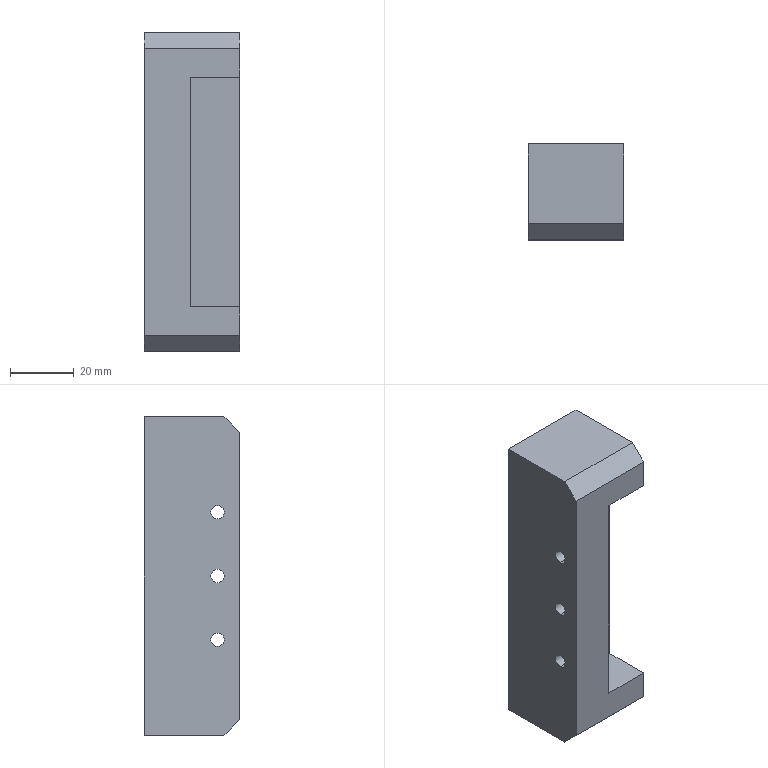Part | SolidWorks | features HoleWzd 2, Chamfer 1, Extrusion 1, ICE 1 | 1 solid | 30 faces | box 30 x 30 x 100 mm | volume 70744 mm3 | cylinder 12 | plane 12 | cone 6 | commonest cylinder face diameters 4.2 x6 6.8 x6
STEP:
#1=CARTESIAN_POINT('',(0.,-8.,22.1));
#2=VERTEX_POINT('',#1);
#3=CARTESIAN_POINT('',(0.,-8.,17.9));
#4=VERTEX_POINT('',#3);
#5=CARTESIAN_POINT('',(0.,-8.,20.));
#6=DIRECTION('',(1.,0.,0.));
#7=DIRECTION('',(0.,0.,-1.));
#8=AXIS2_PLACEMENT_3D('',#5,#6,#7);
#9=CIRCLE('',#8,2.1);
#10=EDGE_CURVE('',#2,#4,#9,.T.);
#11=ORIENTED_EDGE('',*,*,#10,.F.);
#12=CARTESIAN_POINT('',(14.5,-8.,22.1));
#13=VERTEX_POINT('',#12);
#14=CARTESIAN_POINT('',(14.5,-8.,22.1));
#15=DIRECTION('',(1.,0.,0.));
#16=VECTOR('',#15,1000.);
#17=LINE('',#14,#16);
#18=EDGE_CURVE('',#2,#13,#17,.T.);
#19=ORIENTED_EDGE('',*,*,#18,.T.);
#20=CARTESIAN_POINT('',(14.5,-8.,17.9));
#21=VERTEX_POINT('',#20);
#22=CARTESIAN_POINT('',(14.5,-8.,20.));
#23=DIRECTION('',(1.,0.,0.));
#24=DIRECTION('',(0.,0.,-1.));
#25=AXIS2_PLACEMENT_3D('',#22,#23,#24);
#26=CIRCLE('',#25,2.1);
#27=EDGE_CURVE('',#13,#21,#26,.T.);
#28=ORIENTED_EDGE('',*,*,#27,.T.);
#29=CARTESIAN_POINT('',(14.5,-8.,17.9));
#30=DIRECTION('',(1.,0.,0.));
#31=VECTOR('',#30,1000.);
#32=LINE('',#29,#31);
#33=EDGE_CURVE('',#4,#21,#32,.T.);
#34=ORIENTED_EDGE('',*,*,#33,.F.);
#35=EDGE_LOOP('',(#11,#19,#28,#34));
#36=FACE_OUTER_BOUND('',#35,.T.);
#37=CARTESIAN_POINT('',(14.5,-8.,20.));
#38=DIRECTION('',(1.,0.,0.));
#39=DIRECTION('',(0.,0.,-1.));
#40=AXIS2_PLACEMENT_3D('',#37,#38,#39);
#41=CYLINDRICAL_SURFACE('',#40,2.1);
#42=ADVANCED_FACE('',(#36),#41,.F.);
#43=CARTESIAN_POINT('',(0.,-8.,2.1));
#44=VERTEX_POINT('',#43);
#45=CARTESIAN_POINT('',(0.,-8.,-2.1));
#46=VERTEX_POINT('',#45);
#47=CARTESIAN_POINT('',(0.,-8.,0.));
#48=DIRECTION('',(1.,0.,0.));
#49=DIRECTION('',(0.,0.,-1.));
#50=AXIS2_PLACEMENT_3D('',#47,#48,#49);
#51=CIRCLE('',#50,2.1);
#52=EDGE_CURVE('',#44,#46,#51,.T.);
#53=ORIENTED_EDGE('',*,*,#52,.F.);
#54=CARTESIAN_POINT('',(14.5,-8.,2.1));
#55=VERTEX_POINT('',#54);
#56=CARTESIAN_POINT('',(14.5,-8.,2.1));
#57=DIRECTION('',(1.,0.,0.));
#58=VECTOR('',#57,1000.);
#59=LINE('',#56,#58);
#60=EDGE_CURVE('',#44,#55,#59,.T.);
#61=ORIENTED_EDGE('',*,*,#60,.T.);
#62=CARTESIAN_POINT('',(14.5,-8.,-2.1));
#63=VERTEX_POINT('',#62);
#64=CARTESIAN_POINT('',(14.5,-8.,0.));
#65=DIRECTION('',(1.,0.,0.));
#66=DIRECTION('',(0.,0.,-1.));
#67=AXIS2_PLACEMENT_3D('',#64,#65,#66);
#68=CIRCLE('',#67,2.1);
#69=EDGE_CURVE('',#55,#63,#68,.T.);
#70=ORIENTED_EDGE('',*,*,#69,.T.);
#71=CARTESIAN_POINT('',(14.5,-8.,-2.1));
#72=DIRECTION('',(1.,0.,0.));
#73=VECTOR('',#72,1000.);
#74=LINE('',#71,#73);
#75=EDGE_CURVE('',#46,#63,#74,.T.);
#76=ORIENTED_EDGE('',*,*,#75,.F.);
#77=EDGE_LOOP('',(#53,#61,#70,#76));
#78=FACE_OUTER_BOUND('',#77,.T.);
#79=CARTESIAN_POINT('',(14.5,-8.,0.));
#80=DIRECTION('',(1.,0.,0.));
#81=DIRECTION('',(0.,0.,-1.));
#82=AXIS2_PLACEMENT_3D('',#79,#80,#81);
#83=CYLINDRICAL_SURFACE('',#82,2.1);
#84=ADVANCED_FACE('',(#78),#83,.F.);
#85=CARTESIAN_POINT('',(0.,-8.,-17.9));
#86=VERTEX_POINT('',#85);
#87=CARTESIAN_POINT('',(0.,-8.,-22.1));
#88=VERTEX_POINT('',#87);
#89=CARTESIAN_POINT('',(0.,-8.,-20.));
#90=DIRECTION('',(1.,0.,0.));
#91=DIRECTION('',(0.,0.,-1.));
#92=AXIS2_PLACEMENT_3D('',#89,#90,#91);
#93=CIRCLE('',#92,2.1);
#94=EDGE_CURVE('',#86,#88,#93,.T.);
#95=ORIENTED_EDGE('',*,*,#94,.F.);
#96=CARTESIAN_POINT('',(14.5,-8.,-17.9));
#97=VERTEX_POINT('',#96);
#98=CARTESIAN_POINT('',(14.5,-8.,-17.9));
#99=DIRECTION('',(1.,0.,0.));
#100=VECTOR('',#99,1000.);
#101=LINE('',#98,#100);
#102=EDGE_CURVE('',#86,#97,#101,.T.);
#103=ORIENTED_EDGE('',*,*,#102,.T.);
#104=CARTESIAN_POINT('',(14.5,-8.,-22.1));
#105=VERTEX_POINT('',#104);
#106=CARTESIAN_POINT('',(14.5,-8.,-20.));
#107=DIRECTION('',(1.,0.,0.));
#108=DIRECTION('',(0.,0.,-1.));
#109=AXIS2_PLACEMENT_3D('',#106,#107,#108);
#110=CIRCLE('',#109,2.1);
#111=EDGE_CURVE('',#97,#105,#110,.T.);
#112=ORIENTED_EDGE('',*,*,#111,.T.);
#113=CARTESIAN_POINT('',(14.5,-8.,-22.1));
#114=DIRECTION('',(1.,0.,0.));
#115=VECTOR('',#114,1000.);
#116=LINE('',#113,#115);
#117=EDGE_CURVE('',#88,#105,#116,.T.);
#118=ORIENTED_EDGE('',*,*,#117,.F.);
#119=EDGE_LOOP('',(#95,#103,#112,#118));
#120=FACE_OUTER_BOUND('',#119,.T.);
#121=CARTESIAN_POINT('',(14.5,-8.,-20.));
#122=DIRECTION('',(1.,0.,0.));
#123=DIRECTION('',(0.,0.,-1.));
#124=AXIS2_PLACEMENT_3D('',#121,#122,#123);
#125=CYLINDRICAL_SURFACE('',#124,2.1);
#126=ADVANCED_FACE('',(#120),#125,.F.);
#127=CARTESIAN_POINT('',(15.,5.,-3.4));
#128=VERTEX_POINT('',#127);
#129=CARTESIAN_POINT('',(15.,5.,3.4));
#130=VERTEX_POINT('',#129);
#131=CARTESIAN_POINT('',(15.,5.,0.));
#132=DIRECTION('',(0.,1.,0.));
#133=DIRECTION('',(0.,0.,1.));
#134=AXIS2_PLACEMENT_3D('',#131,#132,#133);
#135=CIRCLE('',#134,3.4);
#136=EDGE_CURVE('',#128,#130,#135,.T.);
#137=ORIENTED_EDGE('',*,*,#136,.F.);
#138=CARTESIAN_POINT('',(15.,15.,-3.4));
#139=VERTEX_POINT('',#138);
#140=CARTESIAN_POINT('',(15.,15.,-3.4));
#141=DIRECTION('',(0.,1.,0.));
#142=VECTOR('',#141,1000.);
#143=LINE('',#140,#142);
#144=EDGE_CURVE('',#128,#139,#143,.T.);
#145=ORIENTED_EDGE('',*,*,#144,.T.);
#146=CARTESIAN_POINT('',(15.,15.,3.4));
#147=VERTEX_POINT('',#146);
#148=CARTESIAN_POINT('',(15.,15.,0.));
#149=DIRECTION('',(0.,1.,0.));
#150=DIRECTION('',(0.,0.,1.));
#151=AXIS2_PLACEMENT_3D('',#148,#149,#150);
#152=CIRCLE('',#151,3.4);
#153=EDGE_CURVE('',#139,#147,#152,.T.);
#154=ORIENTED_EDGE('',*,*,#153,.T.);
#155=CARTESIAN_POINT('',(15.,15.,3.4));
#156=DIRECTION('',(0.,1.,0.));
#157=VECTOR('',#156,1000.);
#158=LINE('',#155,#157);
#159=EDGE_CURVE('',#130,#147,#158,.T.);
#160=ORIENTED_EDGE('',*,*,#159,.F.);
#161=EDGE_LOOP('',(#137,#145,#154,#160));
#162=FACE_OUTER_BOUND('',#161,.T.);
#163=CARTESIAN_POINT('',(15.,15.,0.));
#164=DIRECTION('',(0.,1.,0.));
#165=DIRECTION('',(0.,0.,1.));
#166=AXIS2_PLACEMENT_3D('',#163,#164,#165);
#167=CYLINDRICAL_SURFACE('',#166,3.4);
#168=ADVANCED_FACE('',(#162),#167,.F.);
#169=CARTESIAN_POINT('',(15.,2.957,0.));
#170=VERTEX_POINT('',#169);
#171=CARTESIAN_POINT('',(15.,5.,3.4));
#172=DIRECTION('',(0.,0.515,0.8572));
#173=VECTOR('',#172,1000.);
#174=LINE('',#171,#173);
#175=EDGE_CURVE('',#170,#130,#174,.T.);
#176=ORIENTED_EDGE('',*,*,#175,.F.);
#177=CARTESIAN_POINT('',(15.,5.,-3.4));
#178=DIRECTION('',(0.,0.515,-0.8572));
#179=VECTOR('',#178,1000.);
#180=LINE('',#177,#179);
#181=EDGE_CURVE('',#170,#128,#180,.T.);
#182=ORIENTED_EDGE('',*,*,#181,.T.);
#183=ORIENTED_EDGE('',*,*,#136,.T.);
#184=EDGE_LOOP('',(#176,#182,#183));
#185=FACE_OUTER_BOUND('',#184,.T.);
#186=CARTESIAN_POINT('',(15.,5.,0.));
#187=DIRECTION('',(0.,1.,0.));
#188=DIRECTION('',(0.,0.,1.));
#189=AXIS2_PLACEMENT_3D('',#186,#187,#188);
#190=CONICAL_SURFACE('',#189,3.4,1.03);
#191=ADVANCED_FACE('',(#185),#190,.F.);
#192=CARTESIAN_POINT('',(15.,5.,-28.4));
#193=VERTEX_POINT('',#192);
#194=CARTESIAN_POINT('',(15.,5.,-21.6));
#195=VERTEX_POINT('',#194);
#196=CARTESIAN_POINT('',(15.,5.,-25.));
#197=DIRECTION('',(0.,1.,0.));
#198=DIRECTION('',(0.,0.,1.));
#199=AXIS2_PLACEMENT_3D('',#196,#197,#198);
#200=CIRCLE('',#199,3.4);
#201=EDGE_CURVE('',#193,#195,#200,.T.);
#202=ORIENTED_EDGE('',*,*,#201,.F.);
#203=CARTESIAN_POINT('',(15.,15.,-28.4));
#204=VERTEX_POINT('',#203);
#205=CARTESIAN_POINT('',(15.,15.,-28.4));
#206=DIRECTION('',(0.,1.,0.));
#207=VECTOR('',#206,1000.);
#208=LINE('',#205,#207);
#209=EDGE_CURVE('',#193,#204,#208,.T.);
#210=ORIENTED_EDGE('',*,*,#209,.T.);
#211=CARTESIAN_POINT('',(15.,15.,-21.6));
#212=VERTEX_POINT('',#211);
#213=CARTESIAN_POINT('',(15.,15.,-25.));
#214=DIRECTION('',(0.,1.,0.));
#215=DIRECTION('',(0.,0.,1.));
#216=AXIS2_PLACEMENT_3D('',#213,#214,#215);
#217=CIRCLE('',#216,3.4);
#218=EDGE_CURVE('',#204,#212,#217,.T.);
#219=ORIENTED_EDGE('',*,*,#218,.T.);
#220=CARTESIAN_POINT('',(15.,15.,-21.6));
#221=DIRECTION('',(0.,1.,0.));
#222=VECTOR('',#221,1000.);
#223=LINE('',#220,#222);
#224=EDGE_CURVE('',#195,#212,#223,.T.);
#225=ORIENTED_EDGE('',*,*,#224,.F.);
#226=EDGE_LOOP('',(#202,#210,#219,#225));
#227=FACE_OUTER_BOUND('',#226,.T.);
#228=CARTESIAN_POINT('',(15.,15.,-25.));
#229=DIRECTION('',(0.,1.,0.));
#230=DIRECTION('',(0.,0.,1.));
#231=AXIS2_PLACEMENT_3D('',#228,#229,#230);
#232=CYLINDRICAL_SURFACE('',#231,3.4);
#233=ADVANCED_FACE('',(#227),#232,.F.);
#234=CARTESIAN_POINT('',(15.,2.957,-25.));
#235=VERTEX_POINT('',#234);
#236=CARTESIAN_POINT('',(15.,5.,-21.6));
#237=DIRECTION('',(0.,0.515,0.8572));
#238=VECTOR('',#237,1000.);
#239=LINE('',#236,#238);
#240=EDGE_CURVE('',#235,#195,#239,.T.);
#241=ORIENTED_EDGE('',*,*,#240,.F.);
#242=CARTESIAN_POINT('',(15.,5.,-28.4));
#243=DIRECTION('',(0.,0.515,-0.8572));
#244=VECTOR('',#243,1000.);
#245=LINE('',#242,#244);
#246=EDGE_CURVE('',#235,#193,#245,.T.);
#247=ORIENTED_EDGE('',*,*,#246,.T.);
#248=ORIENTED_EDGE('',*,*,#201,.T.);
#249=EDGE_LOOP('',(#241,#247,#248));
#250=FACE_OUTER_BOUND('',#249,.T.);
#251=CARTESIAN_POINT('',(15.,5.,-25.));
#252=DIRECTION('',(0.,1.,0.));
#253=DIRECTION('',(0.,0.,1.));
#254=AXIS2_PLACEMENT_3D('',#251,#252,#253);
#255=CONICAL_SURFACE('',#254,3.4,1.03);
#256=ADVANCED_FACE('',(#250),#255,.F.);
#257=CARTESIAN_POINT('',(15.,5.,21.6));
#258=VERTEX_POINT('',#257);
#259=CARTESIAN_POINT('',(15.,5.,28.4));
#260=VERTEX_POINT('',#259);
#261=CARTESIAN_POINT('',(15.,5.,25.));
#262=DIRECTION('',(0.,1.,0.));
#263=DIRECTION('',(0.,0.,1.));
#264=AXIS2_PLACEMENT_3D('',#261,#262,#263);
#265=CIRCLE('',#264,3.4);
#266=EDGE_CURVE('',#258,#260,#265,.T.);
#267=ORIENTED_EDGE('',*,*,#266,.F.);
#268=CARTESIAN_POINT('',(15.,15.,21.6));
#269=VERTEX_POINT('',#268);
#270=CARTESIAN_POINT('',(15.,15.,21.6));
#271=DIRECTION('',(0.,1.,0.));
#272=VECTOR('',#271,1000.);
#273=LINE('',#270,#272);
#274=EDGE_CURVE('',#258,#269,#273,.T.);
#275=ORIENTED_EDGE('',*,*,#274,.T.);
#276=CARTESIAN_POINT('',(15.,15.,28.4));
#277=VERTEX_POINT('',#276);
#278=CARTESIAN_POINT('',(15.,15.,25.));
#279=DIRECTION('',(0.,1.,0.));
#280=DIRECTION('',(0.,0.,1.));
#281=AXIS2_PLACEMENT_3D('',#278,#279,#280);
#282=CIRCLE('',#281,3.4);
#283=EDGE_CURVE('',#269,#277,#282,.T.);
#284=ORIENTED_EDGE('',*,*,#283,.T.);
#285=CARTESIAN_POINT('',(15.,15.,28.4));
#286=DIRECTION('',(0.,1.,0.));
#287=VECTOR('',#286,1000.);
#288=LINE('',#285,#287);
#289=EDGE_CURVE('',#260,#277,#288,.T.);
#290=ORIENTED_EDGE('',*,*,#289,.F.);
#291=EDGE_LOOP('',(#267,#275,#284,#290));
#292=FACE_OUTER_BOUND('',#291,.T.);
#293=CARTESIAN_POINT('',(15.,15.,25.));
#294=DIRECTION('',(0.,1.,0.));
#295=DIRECTION('',(0.,0.,1.));
#296=AXIS2_PLACEMENT_3D('',#293,#294,#295);
#297=CYLINDRICAL_SURFACE('',#296,3.4);
#298=ADVANCED_FACE('',(#292),#297,.F.);
#299=CARTESIAN_POINT('',(15.,2.957,25.));
#300=VERTEX_POINT('',#299);
#301=CARTESIAN_POINT('',(15.,5.,28.4));
#302=DIRECTION('',(0.,0.515,0.8572));
#303=VECTOR('',#302,1000.);
#304=LINE('',#301,#303);
#305=EDGE_CURVE('',#300,#260,#304,.T.);
#306=ORIENTED_EDGE('',*,*,#305,.F.);
#307=CARTESIAN_POINT('',(15.,5.,21.6));
#308=DIRECTION('',(0.,0.515,-0.8572));
#309=VECTOR('',#308,1000.);
#310=LINE('',#307,#309);
#311=EDGE_CURVE('',#300,#258,#310,.T.);
#312=ORIENTED_EDGE('',*,*,#311,.T.);
#313=ORIENTED_EDGE('',*,*,#266,.T.);
#314=EDGE_LOOP('',(#306,#312,#313));
#315=FACE_OUTER_BOUND('',#314,.T.);
#316=CARTESIAN_POINT('',(15.,5.,25.));
#317=DIRECTION('',(0.,1.,0.));
#318=DIRECTION('',(0.,0.,1.));
#319=AXIS2_PLACEMENT_3D('',#316,#317,#318);
#320=CONICAL_SURFACE('',#319,3.4,1.03);
#321=ADVANCED_FACE('',(#315),#320,.F.);
#322=CARTESIAN_POINT('',(30.,-10.,-50.));
#323=VERTEX_POINT('',#322);
#324=CARTESIAN_POINT('',(30.,15.,-50.));
#325=VERTEX_POINT('',#324);
#326=CARTESIAN_POINT('',(30.,15.,-50.));
#327=DIRECTION('',(0.,1.,0.));
#328=VECTOR('',#327,1000.);
#329=LINE('',#326,#328);
#330=EDGE_CURVE('',#323,#325,#329,.T.);
#331=ORIENTED_EDGE('',*,*,#330,.F.);
#332=CARTESIAN_POINT('',(0.,-10.,-50.));
#333=VERTEX_POINT('',#332);
#334=CARTESIAN_POINT('',(30.,-10.,-50.));
#335=DIRECTION('',(-1.,0.,0.));
#336=VECTOR('',#335,1000.);
#337=LINE('',#334,#336);
#338=EDGE_CURVE('',#323,#333,#337,.T.);
#339=ORIENTED_EDGE('',*,*,#338,.T.);
#340=CARTESIAN_POINT('',(0.,15.,-50.));
#341=VERTEX_POINT('',#340);
#342=CARTESIAN_POINT('',(0.,15.,-50.));
#343=DIRECTION('',(0.,1.,0.));
#344=VECTOR('',#343,1000.);
#345=LINE('',#342,#344);
#346=EDGE_CURVE('',#333,#341,#345,.T.);
#347=ORIENTED_EDGE('',*,*,#346,.T.);
#348=CARTESIAN_POINT('',(30.,15.,-50.));
#349=DIRECTION('',(-1.,0.,0.));
#350=VECTOR('',#349,1000.);
#351=LINE('',#348,#350);
#352=EDGE_CURVE('',#325,#341,#351,.T.);
#353=ORIENTED_EDGE('',*,*,#352,.F.);
#354=EDGE_LOOP('',(#331,#339,#347,#353));
#355=FACE_OUTER_BOUND('',#354,.T.);
#356=CARTESIAN_POINT('',(30.,15.,-50.));
#357=DIRECTION('',(0.,0.,1.));
#358=DIRECTION('',(0.,-1.,0.));
#359=AXIS2_PLACEMENT_3D('',#356,#357,#358);
#360=PLANE('',#359);
#361=ADVANCED_FACE('',(#355),#360,.F.);
#362=CARTESIAN_POINT('',(15.,15.,0.));
#363=DIRECTION('',(0.,1.,0.));
#364=DIRECTION('',(0.,0.,1.));
#365=AXIS2_PLACEMENT_3D('',#362,#363,#364);
#366=CIRCLE('',#365,3.4);
#367=EDGE_CURVE('',#147,#139,#366,.T.);
#368=ORIENTED_EDGE('',*,*,#367,.F.);
#369=ORIENTED_EDGE('',*,*,#153,.F.);
#370=EDGE_LOOP('',(#368,#369));
#371=FACE_BOUND('',#370,.T.);
#372=CARTESIAN_POINT('',(15.,15.,-25.));
#373=DIRECTION('',(0.,1.,0.));
#374=DIRECTION('',(0.,0.,1.));
#375=AXIS2_PLACEMENT_3D('',#372,#373,#374);
#376=CIRCLE('',#375,3.4);
#377=EDGE_CURVE('',#212,#204,#376,.T.);
#378=ORIENTED_EDGE('',*,*,#377,.F.);
#379=ORIENTED_EDGE('',*,*,#218,.F.);
#380=EDGE_LOOP('',(#378,#379));
#381=FACE_BOUND('',#380,.T.);
#382=CARTESIAN_POINT('',(15.,15.,25.));
#383=DIRECTION('',(0.,1.,0.));
#384=DIRECTION('',(0.,0.,1.));
#385=AXIS2_PLACEMENT_3D('',#382,#383,#384);
#386=CIRCLE('',#385,3.4);
#387=EDGE_CURVE('',#277,#269,#386,.T.);
#388=ORIENTED_EDGE('',*,*,#387,.F.);
#389=ORIENTED_EDGE('',*,*,#283,.F.);
#390=EDGE_LOOP('',(#388,#389));
#391=FACE_BOUND('',#390,.T.);
#392=CARTESIAN_POINT('',(0.,15.,50.));
#393=VERTEX_POINT('',#392);
#394=CARTESIAN_POINT('',(0.,15.,50.));
#395=DIRECTION('',(0.,0.,1.));
#396=VECTOR('',#395,1000.);
#397=LINE('',#394,#396);
#398=EDGE_CURVE('',#341,#393,#397,.T.);
#399=ORIENTED_EDGE('',*,*,#398,.T.);
#400=CARTESIAN_POINT('',(30.,15.,50.));
#401=VERTEX_POINT('',#400);
#402=CARTESIAN_POINT('',(30.,15.,50.));
#403=DIRECTION('',(-1.,0.,0.));
#404=VECTOR('',#403,1000.);
#405=LINE('',#402,#404);
#406=EDGE_CURVE('',#401,#393,#405,.T.);
#407=ORIENTED_EDGE('',*,*,#406,.F.);
#408=CARTESIAN_POINT('',(30.,15.,50.));
#409=DIRECTION('',(0.,0.,1.));
#410=VECTOR('',#409,1000.);
#411=LINE('',#408,#410);
#412=EDGE_CURVE('',#325,#401,#411,.T.);
#413=ORIENTED_EDGE('',*,*,#412,.F.);
#414=ORIENTED_EDGE('',*,*,#352,.T.);
#415=EDGE_LOOP('',(#399,#407,#413,#414));
#416=FACE_OUTER_BOUND('',#415,.T.);
#417=CARTESIAN_POINT('',(30.,15.,50.));
#418=DIRECTION('',(0.,-1.,0.));
#419=DIRECTION('',(0.,0.,-1.));
#420=AXIS2_PLACEMENT_3D('',#417,#418,#419);
#421=PLANE('',#420);
#422=ADVANCED_FACE('',(#371,#381,#391,#416),#421,.F.);
#423=CARTESIAN_POINT('',(0.,-10.,50.));
#424=VERTEX_POINT('',#423);
#425=CARTESIAN_POINT('',(0.,15.,50.));
#426=DIRECTION('',(0.,-1.,0.));
#427=VECTOR('',#426,1000.);
#428=LINE('',#425,#427);
#429=EDGE_CURVE('',#393,#424,#428,.T.);
#430=ORIENTED_EDGE('',*,*,#429,.T.);
#431=CARTESIAN_POINT('',(30.,-10.,50.));
#432=VERTEX_POINT('',#431);
#433=CARTESIAN_POINT('',(30.,-10.,50.));
#434=DIRECTION('',(1.,0.,0.));
#435=VECTOR('',#434,1000.);
#436=LINE('',#433,#435);
#437=EDGE_CURVE('',#424,#432,#436,.T.);
#438=ORIENTED_EDGE('',*,*,#437,.T.);
#439=CARTESIAN_POINT('',(30.,15.,50.));
#440=DIRECTION('',(0.,-1.,0.));
#441=VECTOR('',#440,1000.);
#442=LINE('',#439,#441);
#443=EDGE_CURVE('',#401,#432,#442,.T.);
#444=ORIENTED_EDGE('',*,*,#443,.F.);
#445=ORIENTED_EDGE('',*,*,#406,.T.);
#446=EDGE_LOOP('',(#430,#438,#444,#445));
#447=FACE_OUTER_BOUND('',#446,.T.);
#448=CARTESIAN_POINT('',(30.,15.,50.));
#449=DIRECTION('',(0.,0.,-1.));
#450=DIRECTION('',(0.,1.,0.));
#451=AXIS2_PLACEMENT_3D('',#448,#449,#450);
#452=PLANE('',#451);
#453=ADVANCED_FACE('',(#447),#452,.F.);
#454=CARTESIAN_POINT('',(30.,-15.,45.));
#455=VERTEX_POINT('',#454);
#456=CARTESIAN_POINT('',(30.,-15.,36.));
#457=VERTEX_POINT('',#456);
#458=CARTESIAN_POINT('',(30.,-15.,50.));
#459=DIRECTION('',(0.,0.,-1.));
#460=VECTOR('',#459,1000.);
#461=LINE('',#458,#460);
#462=EDGE_CURVE('',#455,#457,#461,.T.);
#463=ORIENTED_EDGE('',*,*,#462,.F.);
#464=CARTESIAN_POINT('',(0.,-15.,45.));
#465=VERTEX_POINT('',#464);
#466=CARTESIAN_POINT('',(30.,-15.,45.));
#467=DIRECTION('',(-1.,0.,0.));
#468=VECTOR('',#467,1000.);
#469=LINE('',#466,#468);
#470=EDGE_CURVE('',#455,#465,#469,.T.);
#471=ORIENTED_EDGE('',*,*,#470,.T.);
#472=CARTESIAN_POINT('',(0.,-15.,-45.));
#473=VERTEX_POINT('',#472);
#474=CARTESIAN_POINT('',(0.,-15.,50.));
#475=DIRECTION('',(0.,0.,-1.));
#476=VECTOR('',#475,1000.);
#477=LINE('',#474,#476);
#478=EDGE_CURVE('',#465,#473,#477,.T.);
#479=ORIENTED_EDGE('',*,*,#478,.T.);
#480=CARTESIAN_POINT('',(30.,-15.,-45.));
#481=VERTEX_POINT('',#480);
#482=CARTESIAN_POINT('',(30.,-15.,-45.));
#483=DIRECTION('',(1.,0.,0.));
#484=VECTOR('',#483,1000.);
#485=LINE('',#482,#484);
#486=EDGE_CURVE('',#473,#481,#485,.T.);
#487=ORIENTED_EDGE('',*,*,#486,.T.);
#488=CARTESIAN_POINT('',(30.,-15.,-36.));
#489=VERTEX_POINT('',#488);
#490=CARTESIAN_POINT('',(30.,-15.,50.));
#491=DIRECTION('',(0.,0.,-1.));
#492=VECTOR('',#491,1000.);
#493=LINE('',#490,#492);
#494=EDGE_CURVE('',#489,#481,#493,.T.);
#495=ORIENTED_EDGE('',*,*,#494,.F.);
#496=CARTESIAN_POINT('',(14.5,-15.,-36.));
#497=VERTEX_POINT('',#496);
#498=CARTESIAN_POINT('',(14.5,-15.,-36.));
#499=DIRECTION('',(1.,0.,0.));
#500=VECTOR('',#499,1000.);
#501=LINE('',#498,#500);
#502=EDGE_CURVE('',#497,#489,#501,.T.);
#503=ORIENTED_EDGE('',*,*,#502,.F.);
#504=CARTESIAN_POINT('',(14.5,-15.,36.));
#505=VERTEX_POINT('',#504);
#506=CARTESIAN_POINT('',(14.5,-15.,36.));
#507=DIRECTION('',(0.,0.,-1.));
#508=VECTOR('',#507,1000.);
#509=LINE('',#506,#508);
#510=EDGE_CURVE('',#505,#497,#509,.T.);
#511=ORIENTED_EDGE('',*,*,#510,.F.);
#512=CARTESIAN_POINT('',(14.5,-15.,36.));
#513=DIRECTION('',(1.,0.,0.));
#514=VECTOR('',#513,1000.);
#515=LINE('',#512,#514);
#516=EDGE_CURVE('',#505,#457,#515,.T.);
#517=ORIENTED_EDGE('',*,*,#516,.T.);
#518=EDGE_LOOP('',(#463,#471,#479,#487,#495,#503,#511,#517));
#519=FACE_OUTER_BOUND('',#518,.T.);
#520=CARTESIAN_POINT('',(30.,-15.,50.));
#521=DIRECTION('',(0.,1.,0.));
#522=DIRECTION('',(0.,0.,1.));
#523=AXIS2_PLACEMENT_3D('',#520,#521,#522);
#524=PLANE('',#523);
#525=ADVANCED_FACE('',(#519),#524,.F.);
#526=ORIENTED_EDGE('',*,*,#443,.T.);
#527=CARTESIAN_POINT('',(30.,-30.,30.));
#528=DIRECTION('',(0.,-0.7071,-0.7071));
#529=VECTOR('',#528,1000.);
#530=LINE('',#527,#529);
#531=EDGE_CURVE('',#432,#455,#530,.T.);
#532=ORIENTED_EDGE('',*,*,#531,.T.);
#533=ORIENTED_EDGE('',*,*,#462,.T.);
#534=CARTESIAN_POINT('',(30.,0.,36.));
#535=VERTEX_POINT('',#534);
#536=CARTESIAN_POINT('',(30.,-15.,36.));
#537=DIRECTION('',(0.,-1.,0.));
#538=VECTOR('',#537,1000.);
#539=LINE('',#536,#538);
#540=EDGE_CURVE('',#535,#457,#539,.T.);
#541=ORIENTED_EDGE('',*,*,#540,.F.);
#542=CARTESIAN_POINT('',(30.,0.,-36.));
#543=VERTEX_POINT('',#542);
#544=CARTESIAN_POINT('',(30.,0.,36.));
#545=DIRECTION('',(0.,0.,1.));
#546=VECTOR('',#545,1000.);
#547=LINE('',#544,#546);
#548=EDGE_CURVE('',#543,#535,#547,.T.);
#549=ORIENTED_EDGE('',*,*,#548,.F.);
#550=CARTESIAN_POINT('',(30.,-15.,-36.));
#551=DIRECTION('',(0.,1.,0.));
#552=VECTOR('',#551,1000.);
#553=LINE('',#550,#552);
#554=EDGE_CURVE('',#489,#543,#553,.T.);
#555=ORIENTED_EDGE('',*,*,#554,.F.);
#556=ORIENTED_EDGE('',*,*,#494,.T.);
#557=CARTESIAN_POINT('',(30.,-30.,-30.));
#558=DIRECTION('',(0.,0.7071,-0.7071));
#559=VECTOR('',#558,1000.);
#560=LINE('',#557,#559);
#561=EDGE_CURVE('',#481,#323,#560,.T.);
#562=ORIENTED_EDGE('',*,*,#561,.T.);
#563=ORIENTED_EDGE('',*,*,#330,.T.);
#564=ORIENTED_EDGE('',*,*,#412,.T.);
#565=EDGE_LOOP('',(#526,#532,#533,#541,#549,#555,#556,#562,#563,#564));
#566=FACE_OUTER_BOUND('',#565,.T.);
#567=CARTESIAN_POINT('',(30.,0.,0.));
#568=DIRECTION('',(1.,0.,0.));
#569=DIRECTION('',(0.,0.,-1.));
#570=AXIS2_PLACEMENT_3D('',#567,#568,#569);
#571=PLANE('',#570);
#572=ADVANCED_FACE('',(#566),#571,.T.);
#573=CARTESIAN_POINT('',(0.,-8.,20.));
#574=DIRECTION('',(1.,0.,0.));
#575=DIRECTION('',(0.,0.,-1.));
#576=AXIS2_PLACEMENT_3D('',#573,#574,#575);
#577=CIRCLE('',#576,2.1);
#578=EDGE_CURVE('',#4,#2,#577,.T.);
#579=ORIENTED_EDGE('',*,*,#578,.T.);
#580=ORIENTED_EDGE('',*,*,#10,.T.);
#581=EDGE_LOOP('',(#579,#580));
#582=FACE_BOUND('',#581,.T.);
#583=CARTESIAN_POINT('',(0.,-8.,0.));
#584=DIRECTION('',(1.,0.,0.));
#585=DIRECTION('',(0.,0.,-1.));
#586=AXIS2_PLACEMENT_3D('',#583,#584,#585);
#587=CIRCLE('',#586,2.1);
#588=EDGE_CURVE('',#46,#44,#587,.T.);
#589=ORIENTED_EDGE('',*,*,#588,.T.);
#590=ORIENTED_EDGE('',*,*,#52,.T.);
#591=EDGE_LOOP('',(#589,#590));
#592=FACE_BOUND('',#591,.T.);
#593=CARTESIAN_POINT('',(0.,-8.,-20.));
#594=DIRECTION('',(1.,0.,0.));
#595=DIRECTION('',(0.,0.,-1.));
#596=AXIS2_PLACEMENT_3D('',#593,#594,#595);
#597=CIRCLE('',#596,2.1);
#598=EDGE_CURVE('',#88,#86,#597,.T.);
#599=ORIENTED_EDGE('',*,*,#598,.T.);
#600=ORIENTED_EDGE('',*,*,#94,.T.);
#601=EDGE_LOOP('',(#599,#600));
#602=FACE_BOUND('',#601,.T.);
#603=ORIENTED_EDGE('',*,*,#478,.F.);
#604=CARTESIAN_POINT('',(0.,-15.,45.));
#605=DIRECTION('',(0.,0.7071,0.7071));
#606=VECTOR('',#605,1000.);
#607=LINE('',#604,#606);
#608=EDGE_CURVE('',#465,#424,#607,.T.);
#609=ORIENTED_EDGE('',*,*,#608,.T.);
#610=ORIENTED_EDGE('',*,*,#429,.F.);
#611=ORIENTED_EDGE('',*,*,#398,.F.);
#612=ORIENTED_EDGE('',*,*,#346,.F.);
#613=CARTESIAN_POINT('',(0.,-10.,-50.));
#614=DIRECTION('',(0.,-0.7071,0.7071));
#615=VECTOR('',#614,1000.);
#616=LINE('',#613,#615);
#617=EDGE_CURVE('',#333,#473,#616,.T.);
#618=ORIENTED_EDGE('',*,*,#617,.T.);
#619=EDGE_LOOP('',(#603,#609,#610,#611,#612,#618));
#620=FACE_OUTER_BOUND('',#619,.T.);
#621=CARTESIAN_POINT('',(0.,0.,0.));
#622=DIRECTION('',(1.,0.,0.));
#623=DIRECTION('',(0.,0.,-1.));
#624=AXIS2_PLACEMENT_3D('',#621,#622,#623);
#625=PLANE('',#624);
#626=ADVANCED_FACE('',(#582,#592,#602,#620),#625,.F.);
#627=ORIENTED_EDGE('',*,*,#540,.T.);
#628=ORIENTED_EDGE('',*,*,#516,.F.);
#629=CARTESIAN_POINT('',(14.5,0.,36.));
#630=VERTEX_POINT('',#629);
#631=CARTESIAN_POINT('',(14.5,-15.,36.));
#632=DIRECTION('',(0.,-1.,0.));
#633=VECTOR('',#632,1000.);
#634=LINE('',#631,#633);
#635=EDGE_CURVE('',#630,#505,#634,.T.);
#636=ORIENTED_EDGE('',*,*,#635,.F.);
#637=CARTESIAN_POINT('',(14.5,0.,36.));
#638=DIRECTION('',(1.,0.,0.));
#639=VECTOR('',#638,1000.);
#640=LINE('',#637,#639);
#641=EDGE_CURVE('',#630,#535,#640,.T.);
#642=ORIENTED_EDGE('',*,*,#641,.T.);
#643=EDGE_LOOP('',(#627,#628,#636,#642));
#644=FACE_OUTER_BOUND('',#643,.T.);
#645=CARTESIAN_POINT('',(14.5,-15.,36.));
#646=DIRECTION('',(0.,0.,1.));
#647=DIRECTION('',(1.,0.,0.));
#648=AXIS2_PLACEMENT_3D('',#645,#646,#647);
#649=PLANE('',#648);
#650=ADVANCED_FACE('',(#644),#649,.F.);
#651=ORIENTED_EDGE('',*,*,#548,.T.);
#652=ORIENTED_EDGE('',*,*,#641,.F.);
#653=CARTESIAN_POINT('',(14.5,0.,-36.));
#654=VERTEX_POINT('',#653);
#655=CARTESIAN_POINT('',(14.5,0.,36.));
#656=DIRECTION('',(0.,0.,1.));
#657=VECTOR('',#656,1000.);
#658=LINE('',#655,#657);
#659=EDGE_CURVE('',#654,#630,#658,.T.);
#660=ORIENTED_EDGE('',*,*,#659,.F.);
#661=CARTESIAN_POINT('',(14.5,0.,-36.));
#662=DIRECTION('',(1.,0.,0.));
#663=VECTOR('',#662,1000.);
#664=LINE('',#661,#663);
#665=EDGE_CURVE('',#654,#543,#664,.T.);
#666=ORIENTED_EDGE('',*,*,#665,.T.);
#667=EDGE_LOOP('',(#651,#652,#660,#666));
#668=FACE_OUTER_BOUND('',#667,.T.);
#669=CARTESIAN_POINT('',(14.5,0.,36.));
#670=DIRECTION('',(0.,1.,0.));
#671=DIRECTION('',(0.,0.,1.));
#672=AXIS2_PLACEMENT_3D('',#669,#670,#671);
#673=PLANE('',#672);
#674=ADVANCED_FACE('',(#668),#673,.F.);
#675=ORIENTED_EDGE('',*,*,#554,.T.);
#676=ORIENTED_EDGE('',*,*,#665,.F.);
#677=CARTESIAN_POINT('',(14.5,-15.,-36.));
#678=DIRECTION('',(0.,1.,0.));
#679=VECTOR('',#678,1000.);
#680=LINE('',#677,#679);
#681=EDGE_CURVE('',#497,#654,#680,.T.);
#682=ORIENTED_EDGE('',*,*,#681,.F.);
#683=ORIENTED_EDGE('',*,*,#502,.T.);
#684=EDGE_LOOP('',(#675,#676,#682,#683));
#685=FACE_OUTER_BOUND('',#684,.T.);
#686=CARTESIAN_POINT('',(14.5,-15.,-36.));
#687=DIRECTION('',(0.,0.,-1.));
#688=DIRECTION('',(0.,1.,0.));
#689=AXIS2_PLACEMENT_3D('',#686,#687,#688);
#690=PLANE('',#689);
#691=ADVANCED_FACE('',(#685),#690,.F.);
#692=CARTESIAN_POINT('',(14.5,-8.,20.));
#693=DIRECTION('',(1.,0.,0.));
#694=DIRECTION('',(0.,0.,-1.));
#695=AXIS2_PLACEMENT_3D('',#692,#693,#694);
#696=CIRCLE('',#695,2.1);
#697=EDGE_CURVE('',#21,#13,#696,.T.);
#698=ORIENTED_EDGE('',*,*,#697,.F.);
#699=ORIENTED_EDGE('',*,*,#27,.F.);
#700=EDGE_LOOP('',(#698,#699));
#701=FACE_BOUND('',#700,.T.);
#702=CARTESIAN_POINT('',(14.5,-8.,0.));
#703=DIRECTION('',(1.,0.,0.));
#704=DIRECTION('',(0.,0.,-1.));
#705=AXIS2_PLACEMENT_3D('',#702,#703,#704);
#706=CIRCLE('',#705,2.1);
#707=EDGE_CURVE('',#63,#55,#706,.T.);
#708=ORIENTED_EDGE('',*,*,#707,.F.);
#709=ORIENTED_EDGE('',*,*,#69,.F.);
#710=EDGE_LOOP('',(#708,#709));
#711=FACE_BOUND('',#710,.T.);
#712=CARTESIAN_POINT('',(14.5,-8.,-20.));
#713=DIRECTION('',(1.,0.,0.));
#714=DIRECTION('',(0.,0.,-1.));
#715=AXIS2_PLACEMENT_3D('',#712,#713,#714);
#716=CIRCLE('',#715,2.1);
#717=EDGE_CURVE('',#105,#97,#716,.T.);
#718=ORIENTED_EDGE('',*,*,#717,.F.);
#719=ORIENTED_EDGE('',*,*,#111,.F.);
#720=EDGE_LOOP('',(#718,#719));
#721=FACE_BOUND('',#720,.T.);
#722=ORIENTED_EDGE('',*,*,#635,.T.);
#723=ORIENTED_EDGE('',*,*,#510,.T.);
#724=ORIENTED_EDGE('',*,*,#681,.T.);
#725=ORIENTED_EDGE('',*,*,#659,.T.);
#726=EDGE_LOOP('',(#722,#723,#724,#725));
#727=FACE_OUTER_BOUND('',#726,.T.);
#728=CARTESIAN_POINT('',(14.5,0.,0.));
#729=DIRECTION('',(-1.,0.,0.));
#730=DIRECTION('',(0.,0.,1.));
#731=AXIS2_PLACEMENT_3D('',#728,#729,#730);
#732=PLANE('',#731);
#733=ADVANCED_FACE('',(#701,#711,#721,#727),#732,.F.);
#734=ORIENTED_EDGE('',*,*,#311,.F.);
#735=ORIENTED_EDGE('',*,*,#305,.T.);
#736=CARTESIAN_POINT('',(15.,5.,25.));
#737=DIRECTION('',(0.,1.,0.));
#738=DIRECTION('',(0.,0.,1.));
#739=AXIS2_PLACEMENT_3D('',#736,#737,#738);
#740=CIRCLE('',#739,3.4);
#741=EDGE_CURVE('',#260,#258,#740,.T.);
#742=ORIENTED_EDGE('',*,*,#741,.T.);
#743=EDGE_LOOP('',(#734,#735,#742));
#744=FACE_OUTER_BOUND('',#743,.T.);
#745=CARTESIAN_POINT('',(15.,5.,25.));
#746=DIRECTION('',(0.,1.,0.));
#747=DIRECTION('',(0.,0.,1.));
#748=AXIS2_PLACEMENT_3D('',#745,#746,#747);
#749=CONICAL_SURFACE('',#748,3.4,1.03);
#750=ADVANCED_FACE('',(#744),#749,.F.);
#751=ORIENTED_EDGE('',*,*,#274,.F.);
#752=ORIENTED_EDGE('',*,*,#741,.F.);
#753=ORIENTED_EDGE('',*,*,#289,.T.);
#754=ORIENTED_EDGE('',*,*,#387,.T.);
#755=EDGE_LOOP('',(#751,#752,#753,#754));
#756=FACE_OUTER_BOUND('',#755,.T.);
#757=CARTESIAN_POINT('',(15.,15.,25.));
#758=DIRECTION('',(0.,1.,0.));
#759=DIRECTION('',(0.,0.,1.));
#760=AXIS2_PLACEMENT_3D('',#757,#758,#759);
#761=CYLINDRICAL_SURFACE('',#760,3.4);
#762=ADVANCED_FACE('',(#756),#761,.F.);
#763=ORIENTED_EDGE('',*,*,#246,.F.);
#764=ORIENTED_EDGE('',*,*,#240,.T.);
#765=CARTESIAN_POINT('',(15.,5.,-25.));
#766=DIRECTION('',(0.,1.,0.));
#767=DIRECTION('',(0.,0.,1.));
#768=AXIS2_PLACEMENT_3D('',#765,#766,#767);
#769=CIRCLE('',#768,3.4);
#770=EDGE_CURVE('',#195,#193,#769,.T.);
#771=ORIENTED_EDGE('',*,*,#770,.T.);
#772=EDGE_LOOP('',(#763,#764,#771));
#773=FACE_OUTER_BOUND('',#772,.T.);
#774=CARTESIAN_POINT('',(15.,5.,-25.));
#775=DIRECTION('',(0.,1.,0.));
#776=DIRECTION('',(0.,0.,1.));
#777=AXIS2_PLACEMENT_3D('',#774,#775,#776);
#778=CONICAL_SURFACE('',#777,3.4,1.03);
#779=ADVANCED_FACE('',(#773),#778,.F.);
#780=ORIENTED_EDGE('',*,*,#209,.F.);
#781=ORIENTED_EDGE('',*,*,#770,.F.);
#782=ORIENTED_EDGE('',*,*,#224,.T.);
#783=ORIENTED_EDGE('',*,*,#377,.T.);
#784=EDGE_LOOP('',(#780,#781,#782,#783));
#785=FACE_OUTER_BOUND('',#784,.T.);
#786=CARTESIAN_POINT('',(15.,15.,-25.));
#787=DIRECTION('',(0.,1.,0.));
#788=DIRECTION('',(0.,0.,1.));
#789=AXIS2_PLACEMENT_3D('',#786,#787,#788);
#790=CYLINDRICAL_SURFACE('',#789,3.4);
#791=ADVANCED_FACE('',(#785),#790,.F.);
#792=ORIENTED_EDGE('',*,*,#181,.F.);
#793=ORIENTED_EDGE('',*,*,#175,.T.);
#794=CARTESIAN_POINT('',(15.,5.,0.));
#795=DIRECTION('',(0.,1.,0.));
#796=DIRECTION('',(0.,0.,1.));
#797=AXIS2_PLACEMENT_3D('',#794,#795,#796);
#798=CIRCLE('',#797,3.4);
#799=EDGE_CURVE('',#130,#128,#798,.T.);
#800=ORIENTED_EDGE('',*,*,#799,.T.);
#801=EDGE_LOOP('',(#792,#793,#800));
#802=FACE_OUTER_BOUND('',#801,.T.);
#803=CARTESIAN_POINT('',(15.,5.,0.));
#804=DIRECTION('',(0.,1.,0.));
#805=DIRECTION('',(0.,0.,1.));
#806=AXIS2_PLACEMENT_3D('',#803,#804,#805);
#807=CONICAL_SURFACE('',#806,3.4,1.03);
#808=ADVANCED_FACE('',(#802),#807,.F.);
#809=ORIENTED_EDGE('',*,*,#144,.F.);
#810=ORIENTED_EDGE('',*,*,#799,.F.);
#811=ORIENTED_EDGE('',*,*,#159,.T.);
#812=ORIENTED_EDGE('',*,*,#367,.T.);
#813=EDGE_LOOP('',(#809,#810,#811,#812));
#814=FACE_OUTER_BOUND('',#813,.T.);
#815=CARTESIAN_POINT('',(15.,15.,0.));
#816=DIRECTION('',(0.,1.,0.));
#817=DIRECTION('',(0.,0.,1.));
#818=AXIS2_PLACEMENT_3D('',#815,#816,#817);
#819=CYLINDRICAL_SURFACE('',#818,3.4);
#820=ADVANCED_FACE('',(#814),#819,.F.);
#821=ORIENTED_EDGE('',*,*,#102,.F.);
#822=ORIENTED_EDGE('',*,*,#598,.F.);
#823=ORIENTED_EDGE('',*,*,#117,.T.);
#824=ORIENTED_EDGE('',*,*,#717,.T.);
#825=EDGE_LOOP('',(#821,#822,#823,#824));
#826=FACE_OUTER_BOUND('',#825,.T.);
#827=CARTESIAN_POINT('',(14.5,-8.,-20.));
#828=DIRECTION('',(1.,0.,0.));
#829=DIRECTION('',(0.,0.,-1.));
#830=AXIS2_PLACEMENT_3D('',#827,#828,#829);
#831=CYLINDRICAL_SURFACE('',#830,2.1);
#832=ADVANCED_FACE('',(#826),#831,.F.);
#833=ORIENTED_EDGE('',*,*,#60,.F.);
#834=ORIENTED_EDGE('',*,*,#588,.F.);
#835=ORIENTED_EDGE('',*,*,#75,.T.);
#836=ORIENTED_EDGE('',*,*,#707,.T.);
#837=EDGE_LOOP('',(#833,#834,#835,#836));
#838=FACE_OUTER_BOUND('',#837,.T.);
#839=CARTESIAN_POINT('',(14.5,-8.,0.));
#840=DIRECTION('',(1.,0.,0.));
#841=DIRECTION('',(0.,0.,-1.));
#842=AXIS2_PLACEMENT_3D('',#839,#840,#841);
#843=CYLINDRICAL_SURFACE('',#842,2.1);
#844=ADVANCED_FACE('',(#838),#843,.F.);
#845=ORIENTED_EDGE('',*,*,#18,.F.);
#846=ORIENTED_EDGE('',*,*,#578,.F.);
#847=ORIENTED_EDGE('',*,*,#33,.T.);
#848=ORIENTED_EDGE('',*,*,#697,.T.);
#849=EDGE_LOOP('',(#845,#846,#847,#848));
#850=FACE_OUTER_BOUND('',#849,.T.);
#851=CARTESIAN_POINT('',(14.5,-8.,20.));
#852=DIRECTION('',(1.,0.,0.));
#853=DIRECTION('',(0.,0.,-1.));
#854=AXIS2_PLACEMENT_3D('',#851,#852,#853);
#855=CYLINDRICAL_SURFACE('',#854,2.1);
#856=ADVANCED_FACE('',(#850),#855,.F.);
#857=ORIENTED_EDGE('',*,*,#531,.F.);
#858=ORIENTED_EDGE('',*,*,#437,.F.);
#859=ORIENTED_EDGE('',*,*,#608,.F.);
#860=ORIENTED_EDGE('',*,*,#470,.F.);
#861=EDGE_LOOP('',(#857,#858,#859,#860));
#862=FACE_OUTER_BOUND('',#861,.T.);
#863=CARTESIAN_POINT('',(30.,-15.,45.));
#864=DIRECTION('',(0.,0.7071,-0.7071));
#865=DIRECTION('',(-1.,0.,0.));
#866=AXIS2_PLACEMENT_3D('',#863,#864,#865);
#867=PLANE('',#866);
#868=ADVANCED_FACE('',(#862),#867,.F.);
#869=ORIENTED_EDGE('',*,*,#561,.F.);
#870=ORIENTED_EDGE('',*,*,#486,.F.);
#871=ORIENTED_EDGE('',*,*,#617,.F.);
#872=ORIENTED_EDGE('',*,*,#338,.F.);
#873=EDGE_LOOP('',(#869,#870,#871,#872));
#874=FACE_OUTER_BOUND('',#873,.T.);
#875=CARTESIAN_POINT('',(30.,-10.,-50.));
#876=DIRECTION('',(0.,0.7071,0.7071));
#877=DIRECTION('',(-1.,0.,0.));
#878=AXIS2_PLACEMENT_3D('',#875,#876,#877);
#879=PLANE('',#878);
#880=ADVANCED_FACE('',(#874),#879,.F.);
#881=CLOSED_SHELL('',(#42,#84,#126,#168,#191,#233,#256,#298,#321,#361,#422,#453,#525,#572,#626,#650,#674,#691,#733,#750,#762,#779,#791,#808,#820,#832,#844,#856,#868,#880));
#882=MANIFOLD_SOLID_BREP('',#881);
#883=CARTESIAN_POINT('',(0.,0.,0.));
#884=DIRECTION('',(0.,0.,1.));
#885=DIRECTION('',(1.,0.,0.));
#886=AXIS2_PLACEMENT_3D('',#883,#884,#885);
#887=(LENGTH_UNIT()NAMED_UNIT(*)SI_UNIT(.MILLI.,.METRE.));
#888=UNCERTAINTY_MEASURE_WITH_UNIT(LENGTH_MEASURE(0.00001),#887,'','');
#889=(NAMED_UNIT(*)PLANE_ANGLE_UNIT()SI_UNIT($,.RADIAN.));
#890=(NAMED_UNIT(*)SI_UNIT($,.STERADIAN.)SOLID_ANGLE_UNIT());
#891=(GEOMETRIC_REPRESENTATION_CONTEXT(3)GLOBAL_UNCERTAINTY_ASSIGNED_CONTEXT((#888))GLOBAL_UNIT_ASSIGNED_CONTEXT((#887,#889,#890))REPRESENTATION_CONTEXT('',''));
#892=ADVANCED_BREP_SHAPE_REPRESENTATION('',(#882,#886),#891);